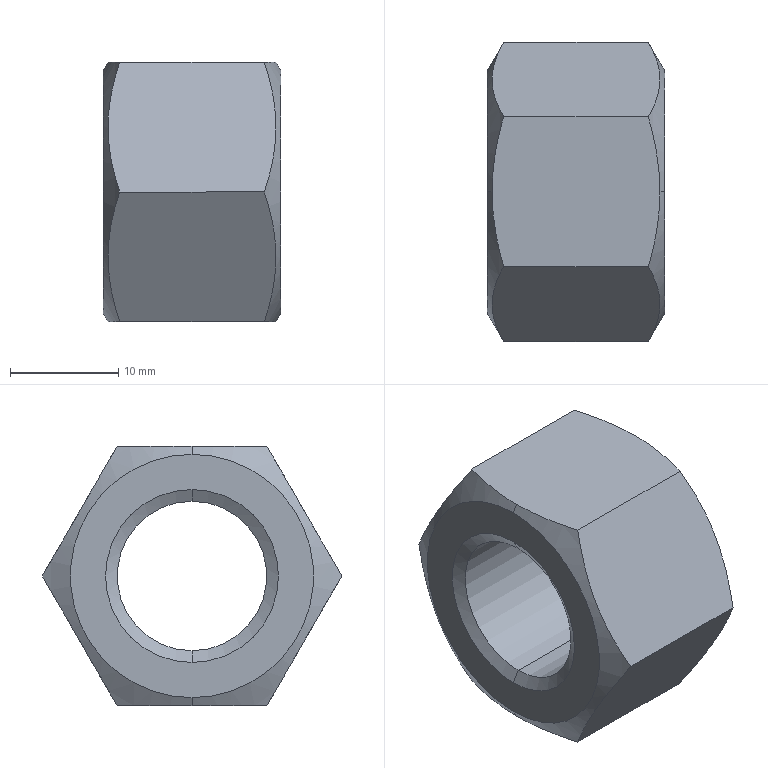Part | STEP file | 1 solid | 18 faces | box 16.4 x 27.713 x 24 mm | volume 5590 mm3 | cone 8 | plane 8 | cylinder 2 | commonest cylinder face diameters 13.835 x2